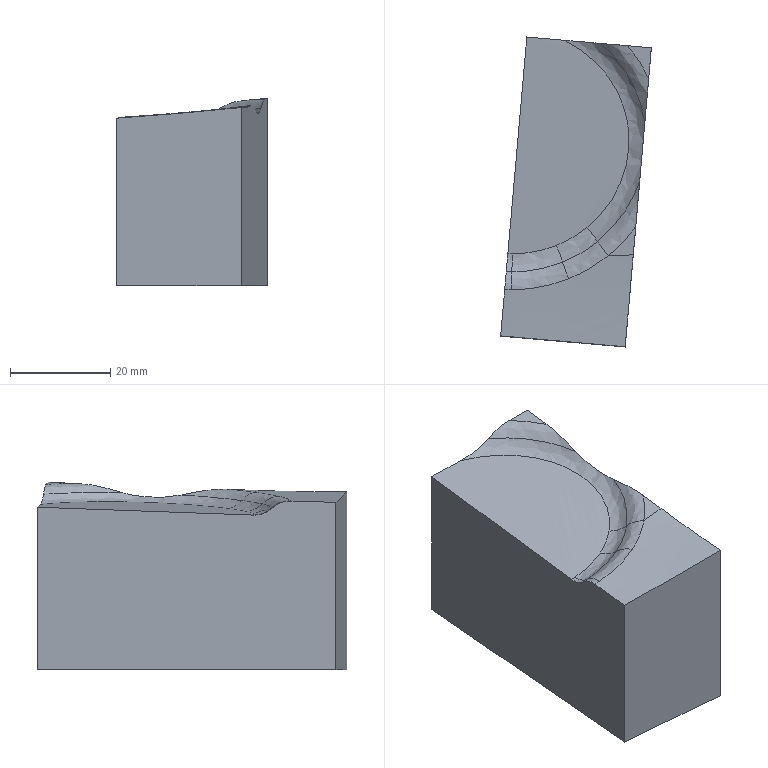Part | NX | features solid 2 | 1 solid | 18 faces | box 30.134 x 61.951 x 37.45 mm | volume 50029 mm3 | spline 13 | plane 5